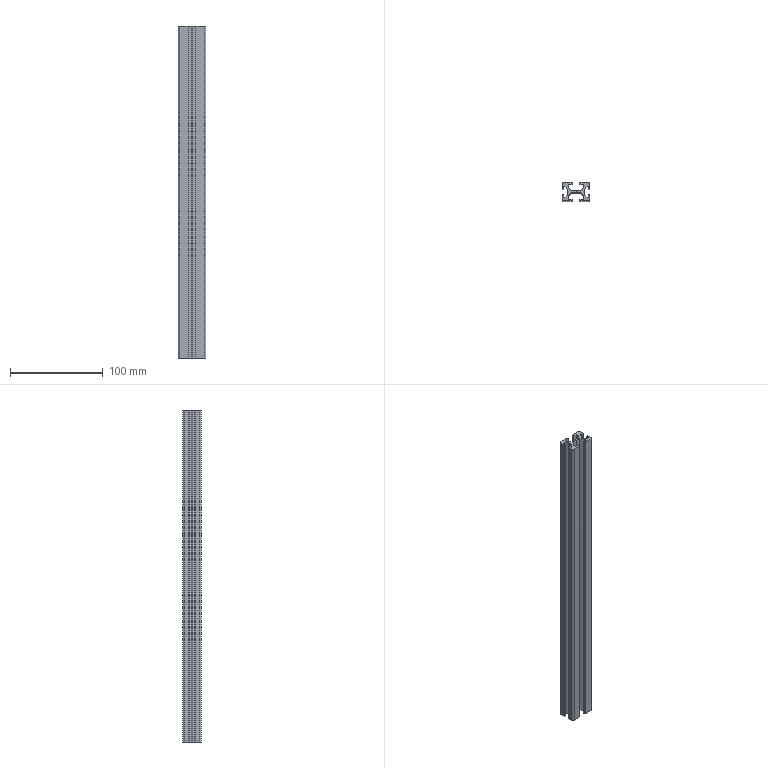Part | STEP file | 11-HFS6-5Y-2030-31511 | 1 solid | 70 faces | box 30 x 20 x 358 mm | volume 90717 mm3 | plane 58 | cylinder 12 | commonest cylinder face diameters 0.6 x8 4 x4